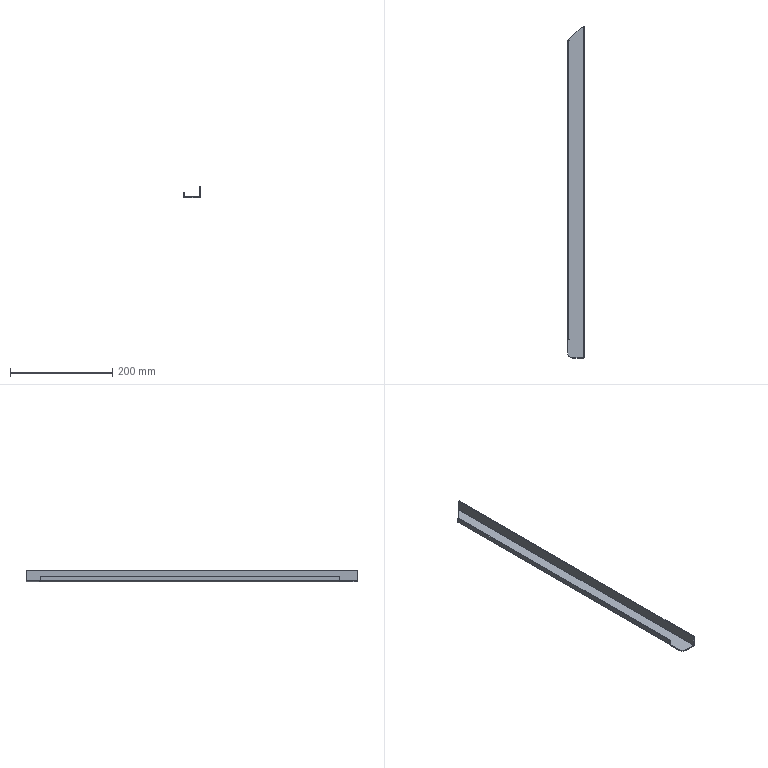Part | STEP file | Rear Closing Plate Door Frame Left | 1 solid | 25 faces | box 32 x 650 x 22 mm | volume 74925 mm3 | plane 17 | cylinder 7 | spline 1 | commonest cylinder face diameters 0.2 x4 4.2 x2 20 x1
STEP:
#1=CARTESIAN_POINT('',(677.249,-292.608,2.));
#2=VERTEX_POINT('',#1);
#3=CARTESIAN_POINT('',(667.249,-282.608,2.));
#4=VERTEX_POINT('',#3);
#5=CARTESIAN_POINT('',(677.249,-282.608,2.));
#6=DIRECTION('',(0.,0.,-1.));
#7=DIRECTION('',(-1.,0.,0.));
#8=AXIS2_PLACEMENT_3D('',#5,#6,#7);
#9=CIRCLE('',#8,10.);
#10=EDGE_CURVE('',#2,#4,#9,.T.);
#11=ORIENTED_EDGE('',*,*,#10,.F.);
#12=CARTESIAN_POINT('',(697.149,-292.608,2.));
#13=VERTEX_POINT('',#12);
#14=CARTESIAN_POINT('',(0.,-292.608,2.));
#15=DIRECTION('',(-1.,0.,0.));
#16=VECTOR('',#15,1000.);
#17=LINE('',#14,#16);
#18=EDGE_CURVE('',#13,#2,#17,.T.);
#19=ORIENTED_EDGE('',*,*,#18,.F.);
#20=CARTESIAN_POINT('',(697.149,357.299,2.));
#21=VERTEX_POINT('',#20);
#22=CARTESIAN_POINT('',(697.149,0.,2.));
#23=DIRECTION('',(0.,-1.,0.));
#24=VECTOR('',#23,1000.);
#25=LINE('',#22,#24);
#26=EDGE_CURVE('',#21,#13,#25,.T.);
#27=ORIENTED_EDGE('',*,*,#26,.F.);
#28=CARTESIAN_POINT('',(669.249,331.392,2.));
#29=VERTEX_POINT('',#28);
#30=CARTESIAN_POINT('',(669.249,331.392,2.));
#31=DIRECTION('',(0.7328,0.6805,0.));
#32=VECTOR('',#31,1000.);
#33=LINE('',#30,#32);
#34=EDGE_CURVE('',#29,#21,#33,.T.);
#35=ORIENTED_EDGE('',*,*,#34,.F.);
#36=CARTESIAN_POINT('',(669.249,329.592,2.));
#37=VERTEX_POINT('',#36);
#38=CARTESIAN_POINT('',(669.249,0.,2.));
#39=DIRECTION('',(0.,1.,0.));
#40=VECTOR('',#39,1000.);
#41=LINE('',#38,#40);
#42=EDGE_CURVE('',#37,#29,#41,.T.);
#43=ORIENTED_EDGE('',*,*,#42,.F.);
#44=CARTESIAN_POINT('',(669.549,329.592,2.));
#45=VERTEX_POINT('',#44);
#46=CARTESIAN_POINT('',(0.,329.592,2.));
#47=DIRECTION('',(-1.,0.,0.));
#48=VECTOR('',#47,1000.);
#49=LINE('',#46,#48);
#50=EDGE_CURVE('',#45,#37,#49,.T.);
#51=ORIENTED_EDGE('',*,*,#50,.F.);
#52=CARTESIAN_POINT('',(669.549,329.392,2.));
#53=VERTEX_POINT('',#52);
#54=CARTESIAN_POINT('',(669.549,329.492,2.));
#55=DIRECTION('',(0.,0.,-1.));
#56=DIRECTION('',(-1.,0.,0.));
#57=AXIS2_PLACEMENT_3D('',#54,#55,#56);
#58=CIRCLE('',#57,0.1);
#59=EDGE_CURVE('',#45,#53,#58,.T.);
#60=ORIENTED_EDGE('',*,*,#59,.T.);
#61=CARTESIAN_POINT('',(669.349,329.392,2.));
#62=VERTEX_POINT('',#61);
#63=CARTESIAN_POINT('',(0.,329.392,2.));
#64=DIRECTION('',(1.,0.,0.));
#65=VECTOR('',#64,1000.);
#66=LINE('',#63,#65);
#67=EDGE_CURVE('',#62,#53,#66,.T.);
#68=ORIENTED_EDGE('',*,*,#67,.F.);
#69=CARTESIAN_POINT('',(669.349,-256.608,2.));
#70=VERTEX_POINT('',#69);
#71=CARTESIAN_POINT('',(669.349,0.,2.));
#72=DIRECTION('',(0.,1.,0.));
#73=VECTOR('',#72,1000.);
#74=LINE('',#71,#73);
#75=EDGE_CURVE('',#70,#62,#74,.T.);
#76=ORIENTED_EDGE('',*,*,#75,.F.);
#77=CARTESIAN_POINT('',(669.549,-256.608,2.));
#78=VERTEX_POINT('',#77);
#79=CARTESIAN_POINT('',(0.,-256.608,2.));
#80=DIRECTION('',(-1.,0.,0.));
#81=VECTOR('',#80,1000.);
#82=LINE('',#79,#81);
#83=EDGE_CURVE('',#78,#70,#82,.T.);
#84=ORIENTED_EDGE('',*,*,#83,.F.);
#85=CARTESIAN_POINT('',(669.549,-256.808,2.));
#86=VERTEX_POINT('',#85);
#87=CARTESIAN_POINT('',(669.549,-256.708,2.));
#88=DIRECTION('',(0.,0.,-1.));
#89=DIRECTION('',(-1.,0.,0.));
#90=AXIS2_PLACEMENT_3D('',#87,#88,#89);
#91=CIRCLE('',#90,0.1);
#92=EDGE_CURVE('',#78,#86,#91,.T.);
#93=ORIENTED_EDGE('',*,*,#92,.T.);
#94=CARTESIAN_POINT('',(667.249,-256.808,2.));
#95=VERTEX_POINT('',#94);
#96=CARTESIAN_POINT('',(0.,-256.808,2.));
#97=DIRECTION('',(1.,0.,0.));
#98=VECTOR('',#97,1000.);
#99=LINE('',#96,#98);
#100=EDGE_CURVE('',#95,#86,#99,.T.);
#101=ORIENTED_EDGE('',*,*,#100,.F.);
#102=CARTESIAN_POINT('',(667.249,0.,2.));
#103=DIRECTION('',(0.,1.,0.));
#104=VECTOR('',#103,1000.);
#105=LINE('',#102,#104);
#106=EDGE_CURVE('',#4,#95,#105,.T.);
#107=ORIENTED_EDGE('',*,*,#106,.F.);
#108=EDGE_LOOP('',(#11,#19,#27,#35,#43,#51,#60,#68,#76,#84,#93,#101,#107));
#109=FACE_OUTER_BOUND('',#108,.T.);
#110=CARTESIAN_POINT('',(0.,0.,2.));
#111=DIRECTION('',(0.,0.,-1.));
#112=DIRECTION('',(-1.,0.,0.));
#113=AXIS2_PLACEMENT_3D('',#110,#111,#112);
#114=PLANE('',#113);
#115=ADVANCED_FACE('',(#109),#114,.F.);
#116=CARTESIAN_POINT('',(667.249,-282.608,0.));
#117=VERTEX_POINT('',#116);
#118=CARTESIAN_POINT('',(667.249,-282.608,1301.189));
#119=DIRECTION('',(0.,0.,-1.));
#120=VECTOR('',#119,1000.);
#121=LINE('',#118,#120);
#122=EDGE_CURVE('',#4,#117,#121,.T.);
#123=ORIENTED_EDGE('',*,*,#122,.F.);
#124=ORIENTED_EDGE('',*,*,#106,.T.);
#125=CARTESIAN_POINT('',(667.249,-256.808,0.));
#126=VERTEX_POINT('',#125);
#127=CARTESIAN_POINT('',(667.249,-256.808,1301.189));
#128=DIRECTION('',(0.,0.,1.));
#129=VECTOR('',#128,1000.);
#130=LINE('',#127,#129);
#131=EDGE_CURVE('',#126,#95,#130,.T.);
#132=ORIENTED_EDGE('',*,*,#131,.F.);
#133=CARTESIAN_POINT('',(667.249,0.,0.));
#134=DIRECTION('',(0.,1.,0.));
#135=VECTOR('',#134,1000.);
#136=LINE('',#133,#135);
#137=EDGE_CURVE('',#117,#126,#136,.T.);
#138=ORIENTED_EDGE('',*,*,#137,.F.);
#139=EDGE_LOOP('',(#123,#124,#132,#138));
#140=FACE_OUTER_BOUND('',#139,.T.);
#141=CARTESIAN_POINT('',(667.249,0.,1301.189));
#142=DIRECTION('',(1.,0.,0.));
#143=DIRECTION('',(0.,0.,-1.));
#144=AXIS2_PLACEMENT_3D('',#141,#142,#143);
#145=PLANE('',#144);
#146=ADVANCED_FACE('',(#140),#145,.F.);
#147=CARTESIAN_POINT('',(677.249,-292.608,0.));
#148=VERTEX_POINT('',#147);
#149=CARTESIAN_POINT('',(677.249,-282.608,0.));
#150=DIRECTION('',(0.,0.,1.));
#151=DIRECTION('',(-1.,0.,0.));
#152=AXIS2_PLACEMENT_3D('',#149,#150,#151);
#153=CIRCLE('',#152,10.);
#154=EDGE_CURVE('',#117,#148,#153,.T.);
#155=ORIENTED_EDGE('',*,*,#154,.T.);
#156=CARTESIAN_POINT('',(677.249,-292.608,1301.189));
#157=DIRECTION('',(0.,0.,1.));
#158=VECTOR('',#157,1000.);
#159=LINE('',#156,#158);
#160=EDGE_CURVE('',#148,#2,#159,.T.);
#161=ORIENTED_EDGE('',*,*,#160,.T.);
#162=ORIENTED_EDGE('',*,*,#10,.T.);
#163=ORIENTED_EDGE('',*,*,#122,.T.);
#164=EDGE_LOOP('',(#155,#161,#162,#163));
#165=FACE_OUTER_BOUND('',#164,.T.);
#166=CARTESIAN_POINT('',(677.249,-282.608,1301.189));
#167=DIRECTION('',(0.,0.,-1.));
#168=DIRECTION('',(-1.,0.,0.));
#169=AXIS2_PLACEMENT_3D('',#166,#167,#168);
#170=CYLINDRICAL_SURFACE('',#169,10.);
#171=ADVANCED_FACE('',(#165),#170,.T.);
#172=ORIENTED_EDGE('',*,*,#160,.F.);
#173=CARTESIAN_POINT('',(697.149,-292.608,0.));
#174=VERTEX_POINT('',#173);
#175=CARTESIAN_POINT('',(0.,-292.608,0.));
#176=DIRECTION('',(-1.,0.,0.));
#177=VECTOR('',#176,1000.);
#178=LINE('',#175,#177);
#179=EDGE_CURVE('',#174,#148,#178,.T.);
#180=ORIENTED_EDGE('',*,*,#179,.F.);
#181=CARTESIAN_POINT('',(699.249,-292.608,2.1));
#182=VERTEX_POINT('',#181);
#183=CARTESIAN_POINT('',(697.149,-292.608,2.1));
#184=DIRECTION('',(0.,-1.,0.));
#185=DIRECTION('',(-1.,0.,0.));
#186=AXIS2_PLACEMENT_3D('',#183,#184,#185);
#187=CIRCLE('',#186,2.1);
#188=EDGE_CURVE('',#174,#182,#187,.T.);
#189=ORIENTED_EDGE('',*,*,#188,.T.);
#190=CARTESIAN_POINT('',(699.249,-292.608,22.));
#191=VERTEX_POINT('',#190);
#192=CARTESIAN_POINT('',(699.249,-292.608,22.));
#193=DIRECTION('',(0.,0.,1.));
#194=VECTOR('',#193,1000.);
#195=LINE('',#192,#194);
#196=EDGE_CURVE('',#182,#191,#195,.T.);
#197=ORIENTED_EDGE('',*,*,#196,.T.);
#198=CARTESIAN_POINT('',(697.249,-292.608,22.));
#199=VERTEX_POINT('',#198);
#200=CARTESIAN_POINT('',(-601.36,-292.608,22.));
#201=DIRECTION('',(-1.,0.,0.));
#202=VECTOR('',#201,1000.);
#203=LINE('',#200,#202);
#204=EDGE_CURVE('',#191,#199,#203,.T.);
#205=ORIENTED_EDGE('',*,*,#204,.T.);
#206=CARTESIAN_POINT('',(697.249,-292.608,2.1));
#207=VERTEX_POINT('',#206);
#208=CARTESIAN_POINT('',(697.249,-292.608,22.));
#209=DIRECTION('',(0.,0.,1.));
#210=VECTOR('',#209,1000.);
#211=LINE('',#208,#210);
#212=EDGE_CURVE('',#207,#199,#211,.T.);
#213=ORIENTED_EDGE('',*,*,#212,.F.);
#214=CARTESIAN_POINT('',(697.149,-292.608,2.1));
#215=DIRECTION('',(0.,1.,0.));
#216=DIRECTION('',(-1.,0.,0.));
#217=AXIS2_PLACEMENT_3D('',#214,#215,#216);
#218=CIRCLE('',#217,0.1);
#219=EDGE_CURVE('',#207,#13,#218,.T.);
#220=ORIENTED_EDGE('',*,*,#219,.T.);
#221=ORIENTED_EDGE('',*,*,#18,.T.);
#222=EDGE_LOOP('',(#172,#180,#189,#197,#205,#213,#220,#221));
#223=FACE_OUTER_BOUND('',#222,.T.);
#224=CARTESIAN_POINT('',(0.,-292.608,1301.189));
#225=DIRECTION('',(0.,1.,0.));
#226=DIRECTION('',(0.,0.,1.));
#227=AXIS2_PLACEMENT_3D('',#224,#225,#226);
#228=PLANE('',#227);
#229=ADVANCED_FACE('',(#223),#228,.F.);
#230=ORIENTED_EDGE('',*,*,#219,.F.);
#231=CARTESIAN_POINT('',(697.249,357.392,2.1));
#232=VERTEX_POINT('',#231);
#233=CARTESIAN_POINT('',(697.249,-945.215,2.1));
#234=DIRECTION('',(0.,-1.,0.));
#235=VECTOR('',#234,1000.);
#236=LINE('',#233,#235);
#237=EDGE_CURVE('',#232,#207,#236,.T.);
#238=ORIENTED_EDGE('',*,*,#237,.F.);
#239=CARTESIAN_POINT('',(697.161,357.392,2.001));
#240=VERTEX_POINT('',#239);
#241=CARTESIAN_POINT('',(697.149,357.392,2.1));
#242=DIRECTION('',(0.,-1.,0.));
#243=DIRECTION('',(-1.,0.,0.));
#244=AXIS2_PLACEMENT_3D('',#241,#242,#243);
#245=CIRCLE('',#244,0.1);
#246=EDGE_CURVE('',#240,#232,#245,.T.);
#247=ORIENTED_EDGE('',*,*,#246,.F.);
#248=CARTESIAN_POINT('',(697.149,357.299,2.));
#249=CARTESIAN_POINT('',(697.153,357.33,2.));
#250=CARTESIAN_POINT('',(697.157,357.361,2.));
#251=CARTESIAN_POINT('',(697.161,357.392,2.001));
#252=B_SPLINE_CURVE_WITH_KNOTS('',3,(#248,#249,#250,#251),.UNSPECIFIED.,.F.,.F.,(4,4),(0.,1.),.UNSPECIFIED.);
#253=EDGE_CURVE('',#21,#240,#252,.T.);
#254=ORIENTED_EDGE('',*,*,#253,.F.);
#255=ORIENTED_EDGE('',*,*,#26,.T.);
#256=EDGE_LOOP('',(#230,#238,#247,#254,#255));
#257=FACE_OUTER_BOUND('',#256,.T.);
#258=CARTESIAN_POINT('',(697.149,-945.215,2.1));
#259=DIRECTION('',(0.,1.,0.));
#260=DIRECTION('',(-1.,0.,0.));
#261=AXIS2_PLACEMENT_3D('',#258,#259,#260);
#262=CYLINDRICAL_SURFACE('',#261,0.1);
#263=ADVANCED_FACE('',(#257),#262,.F.);
#264=CARTESIAN_POINT('',(669.249,331.392,0.));
#265=VERTEX_POINT('',#264);
#266=CARTESIAN_POINT('',(669.249,331.392,1301.189));
#267=DIRECTION('',(0.,0.,-1.));
#268=VECTOR('',#267,1000.);
#269=LINE('',#266,#268);
#270=EDGE_CURVE('',#29,#265,#269,.T.);
#271=ORIENTED_EDGE('',*,*,#270,.F.);
#272=ORIENTED_EDGE('',*,*,#34,.T.);
#273=CARTESIAN_POINT('',(697.149,357.299,0.));
#274=VERTEX_POINT('',#273);
#275=CARTESIAN_POINT('',(697.149,357.299,1301.189));
#276=DIRECTION('',(0.,0.,1.));
#277=VECTOR('',#276,1000.);
#278=LINE('',#275,#277);
#279=EDGE_CURVE('',#274,#21,#278,.T.);
#280=ORIENTED_EDGE('',*,*,#279,.F.);
#281=CARTESIAN_POINT('',(144.63,-155.755,0.));
#282=DIRECTION('',(0.7328,0.6805,0.));
#283=VECTOR('',#282,1000.);
#284=LINE('',#281,#283);
#285=EDGE_CURVE('',#265,#274,#284,.T.);
#286=ORIENTED_EDGE('',*,*,#285,.F.);
#287=EDGE_LOOP('',(#271,#272,#280,#286));
#288=FACE_OUTER_BOUND('',#287,.T.);
#289=CARTESIAN_POINT('',(144.63,-155.755,1301.189));
#290=DIRECTION('',(0.6805,-0.7328,0.));
#291=DIRECTION('',(0.7328,0.6805,0.));
#292=AXIS2_PLACEMENT_3D('',#289,#290,#291);
#293=PLANE('',#292);
#294=ADVANCED_FACE('',(#288),#293,.F.);
#295=CARTESIAN_POINT('',(669.249,329.592,0.));
#296=VERTEX_POINT('',#295);
#297=CARTESIAN_POINT('',(669.249,329.592,1301.189));
#298=DIRECTION('',(0.,0.,-1.));
#299=VECTOR('',#298,1000.);
#300=LINE('',#297,#299);
#301=EDGE_CURVE('',#37,#296,#300,.T.);
#302=ORIENTED_EDGE('',*,*,#301,.F.);
#303=ORIENTED_EDGE('',*,*,#42,.T.);
#304=ORIENTED_EDGE('',*,*,#270,.T.);
#305=CARTESIAN_POINT('',(669.249,0.,0.));
#306=DIRECTION('',(0.,1.,0.));
#307=VECTOR('',#306,1000.);
#308=LINE('',#305,#307);
#309=EDGE_CURVE('',#296,#265,#308,.T.);
#310=ORIENTED_EDGE('',*,*,#309,.F.);
#311=EDGE_LOOP('',(#302,#303,#304,#310));
#312=FACE_OUTER_BOUND('',#311,.T.);
#313=CARTESIAN_POINT('',(669.249,0.,1301.189));
#314=DIRECTION('',(1.,0.,0.));
#315=DIRECTION('',(0.,1.,0.));
#316=AXIS2_PLACEMENT_3D('',#313,#314,#315);
#317=PLANE('',#316);
#318=ADVANCED_FACE('',(#312),#317,.F.);
#319=CARTESIAN_POINT('',(669.249,329.392,2.1));
#320=VERTEX_POINT('',#319);
#321=CARTESIAN_POINT('',(669.349,329.392,2.1));
#322=DIRECTION('',(0.,-1.,0.));
#323=DIRECTION('',(0.,0.,-1.));
#324=AXIS2_PLACEMENT_3D('',#321,#322,#323);
#325=CIRCLE('',#324,0.1);
#326=EDGE_CURVE('',#320,#62,#325,.T.);
#327=ORIENTED_EDGE('',*,*,#326,.F.);
#328=CARTESIAN_POINT('',(669.249,-256.608,2.1));
#329=VERTEX_POINT('',#328);
#330=CARTESIAN_POINT('',(669.249,980.944,2.1));
#331=DIRECTION('',(0.,1.,0.));
#332=VECTOR('',#331,1000.);
#333=LINE('',#330,#332);
#334=EDGE_CURVE('',#329,#320,#333,.T.);
#335=ORIENTED_EDGE('',*,*,#334,.F.);
#336=CARTESIAN_POINT('',(669.349,-256.608,2.1));
#337=DIRECTION('',(0.,1.,0.));
#338=DIRECTION('',(0.,0.,-1.));
#339=AXIS2_PLACEMENT_3D('',#336,#337,#338);
#340=CIRCLE('',#339,0.1);
#341=EDGE_CURVE('',#70,#329,#340,.T.);
#342=ORIENTED_EDGE('',*,*,#341,.F.);
#343=ORIENTED_EDGE('',*,*,#75,.T.);
#344=EDGE_LOOP('',(#327,#335,#342,#343));
#345=FACE_OUTER_BOUND('',#344,.T.);
#346=CARTESIAN_POINT('',(669.349,980.944,2.1));
#347=DIRECTION('',(0.,-1.,0.));
#348=DIRECTION('',(0.,0.,-1.));
#349=AXIS2_PLACEMENT_3D('',#346,#347,#348);
#350=CYLINDRICAL_SURFACE('',#349,0.1);
#351=ADVANCED_FACE('',(#345),#350,.F.);
#352=ORIENTED_EDGE('',*,*,#131,.T.);
#353=ORIENTED_EDGE('',*,*,#100,.T.);
#354=CARTESIAN_POINT('',(669.549,-256.808,0.));
#355=VERTEX_POINT('',#354);
#356=CARTESIAN_POINT('',(669.549,-256.808,1301.189));
#357=DIRECTION('',(0.,0.,-1.));
#358=VECTOR('',#357,1000.);
#359=LINE('',#356,#358);
#360=EDGE_CURVE('',#86,#355,#359,.T.);
#361=ORIENTED_EDGE('',*,*,#360,.T.);
#362=CARTESIAN_POINT('',(0.,-256.808,0.));
#363=DIRECTION('',(-1.,0.,0.));
#364=VECTOR('',#363,1000.);
#365=LINE('',#362,#364);
#366=EDGE_CURVE('',#355,#126,#365,.T.);
#367=ORIENTED_EDGE('',*,*,#366,.T.);
#368=EDGE_LOOP('',(#352,#353,#361,#367));
#369=FACE_OUTER_BOUND('',#368,.T.);
#370=CARTESIAN_POINT('',(0.,-256.808,1301.189));
#371=DIRECTION('',(0.,1.,0.));
#372=DIRECTION('',(0.,0.,1.));
#373=AXIS2_PLACEMENT_3D('',#370,#371,#372);
#374=PLANE('',#373);
#375=ADVANCED_FACE('',(#369),#374,.T.);
#376=ORIENTED_EDGE('',*,*,#285,.T.);
#377=CARTESIAN_POINT('',(697.149,0.,0.));
#378=DIRECTION('',(0.,-1.,0.));
#379=VECTOR('',#378,1000.);
#380=LINE('',#377,#379);
#381=EDGE_CURVE('',#274,#174,#380,.T.);
#382=ORIENTED_EDGE('',*,*,#381,.T.);
#383=ORIENTED_EDGE('',*,*,#179,.T.);
#384=ORIENTED_EDGE('',*,*,#154,.F.);
#385=ORIENTED_EDGE('',*,*,#137,.T.);
#386=ORIENTED_EDGE('',*,*,#366,.F.);
#387=CARTESIAN_POINT('',(669.549,-256.608,0.));
#388=VERTEX_POINT('',#387);
#389=CARTESIAN_POINT('',(669.549,-256.708,0.));
#390=DIRECTION('',(0.,0.,1.));
#391=DIRECTION('',(-1.,0.,0.));
#392=AXIS2_PLACEMENT_3D('',#389,#390,#391);
#393=CIRCLE('',#392,0.1);
#394=EDGE_CURVE('',#355,#388,#393,.T.);
#395=ORIENTED_EDGE('',*,*,#394,.T.);
#396=CARTESIAN_POINT('',(669.349,-256.608,0.));
#397=VERTEX_POINT('',#396);
#398=CARTESIAN_POINT('',(0.,-256.608,0.));
#399=DIRECTION('',(1.,0.,0.));
#400=VECTOR('',#399,1000.);
#401=LINE('',#398,#400);
#402=EDGE_CURVE('',#397,#388,#401,.T.);
#403=ORIENTED_EDGE('',*,*,#402,.F.);
#404=CARTESIAN_POINT('',(669.349,329.392,0.));
#405=VERTEX_POINT('',#404);
#406=CARTESIAN_POINT('',(669.349,0.,0.));
#407=DIRECTION('',(0.,1.,0.));
#408=VECTOR('',#407,1000.);
#409=LINE('',#406,#408);
#410=EDGE_CURVE('',#397,#405,#409,.T.);
#411=ORIENTED_EDGE('',*,*,#410,.T.);
#412=CARTESIAN_POINT('',(669.549,329.392,0.));
#413=VERTEX_POINT('',#412);
#414=CARTESIAN_POINT('',(0.,329.392,0.));
#415=DIRECTION('',(-1.,0.,0.));
#416=VECTOR('',#415,1000.);
#417=LINE('',#414,#416);
#418=EDGE_CURVE('',#413,#405,#417,.T.);
#419=ORIENTED_EDGE('',*,*,#418,.F.);
#420=CARTESIAN_POINT('',(669.549,329.592,0.));
#421=VERTEX_POINT('',#420);
#422=CARTESIAN_POINT('',(669.549,329.492,0.));
#423=DIRECTION('',(0.,0.,1.));
#424=DIRECTION('',(-1.,0.,0.));
#425=AXIS2_PLACEMENT_3D('',#422,#423,#424);
#426=CIRCLE('',#425,0.1);
#427=EDGE_CURVE('',#413,#421,#426,.T.);
#428=ORIENTED_EDGE('',*,*,#427,.T.);
#429=CARTESIAN_POINT('',(0.,329.592,0.));
#430=DIRECTION('',(-1.,0.,0.));
#431=VECTOR('',#430,1000.);
#432=LINE('',#429,#431);
#433=EDGE_CURVE('',#421,#296,#432,.T.);
#434=ORIENTED_EDGE('',*,*,#433,.T.);
#435=ORIENTED_EDGE('',*,*,#309,.T.);
#436=EDGE_LOOP('',(#376,#382,#383,#384,#385,#386,#395,#403,#411,#419,#428,#434,#435));
#437=FACE_OUTER_BOUND('',#436,.T.);
#438=CARTESIAN_POINT('',(0.,0.,0.));
#439=DIRECTION('',(0.,0.,-1.));
#440=DIRECTION('',(-1.,0.,0.));
#441=AXIS2_PLACEMENT_3D('',#438,#439,#440);
#442=PLANE('',#441);
#443=ADVANCED_FACE('',(#437),#442,.T.);
#444=CARTESIAN_POINT('',(697.249,357.392,22.));
#445=VERTEX_POINT('',#444);
#446=CARTESIAN_POINT('',(697.249,359.392,22.));
#447=DIRECTION('',(0.,1.,0.));
#448=VECTOR('',#447,1000.);
#449=LINE('',#446,#448);
#450=EDGE_CURVE('',#199,#445,#449,.T.);
#451=ORIENTED_EDGE('',*,*,#450,.T.);
#452=CARTESIAN_POINT('',(697.249,357.392,22.));
#453=DIRECTION('',(0.,0.,-1.));
#454=VECTOR('',#453,1000.);
#455=LINE('',#452,#454);
#456=EDGE_CURVE('',#445,#232,#455,.T.);
#457=ORIENTED_EDGE('',*,*,#456,.T.);
#458=ORIENTED_EDGE('',*,*,#237,.T.);
#459=ORIENTED_EDGE('',*,*,#212,.T.);
#460=EDGE_LOOP('',(#451,#457,#458,#459));
#461=FACE_OUTER_BOUND('',#460,.T.);
#462=CARTESIAN_POINT('',(697.249,359.392,22.));
#463=DIRECTION('',(-1.,0.,0.));
#464=DIRECTION('',(0.,-1.,0.));
#465=AXIS2_PLACEMENT_3D('',#462,#463,#464);
#466=PLANE('',#465);
#467=ADVANCED_FACE('',(#461),#466,.T.);
#468=CARTESIAN_POINT('',(697.398,357.392,0.01486));
#469=VERTEX_POINT('',#468);
#470=CARTESIAN_POINT('',(697.398,357.392,0.01486));
#471=CARTESIAN_POINT('',(697.316,357.361,0.004966));
#472=CARTESIAN_POINT('',(697.232,357.33,0.));
#473=CARTESIAN_POINT('',(697.149,357.299,0.));
#474=B_SPLINE_CURVE_WITH_KNOTS('',3,(#470,#471,#472,#473),.UNSPECIFIED.,.F.,.F.,(4,4),(0.,1.),.UNSPECIFIED.);
#475=EDGE_CURVE('',#469,#274,#474,.T.);
#476=ORIENTED_EDGE('',*,*,#475,.T.);
#477=ORIENTED_EDGE('',*,*,#279,.T.);
#478=ORIENTED_EDGE('',*,*,#253,.T.);
#479=CARTESIAN_POINT('',(697.279,357.392,1.008));
#480=DIRECTION('',(0.1188,0.,-0.9929));
#481=VECTOR('',#480,1000.);
#482=LINE('',#479,#481);
#483=EDGE_CURVE('',#240,#469,#482,.T.);
#484=ORIENTED_EDGE('',*,*,#483,.T.);
#485=EDGE_LOOP('',(#476,#477,#478,#484));
#486=FACE_OUTER_BOUND('',#485,.T.);
#487=CARTESIAN_POINT('',(697.149,357.299,0.));
#488=CARTESIAN_POINT('',(697.232,357.33,0.));
#489=CARTESIAN_POINT('',(697.316,357.361,0.004966));
#490=CARTESIAN_POINT('',(697.398,357.392,0.01486));
#491=CARTESIAN_POINT('',(697.149,357.299,2.));
#492=CARTESIAN_POINT('',(697.153,357.33,2.));
#493=CARTESIAN_POINT('',(697.157,357.361,2.));
#494=CARTESIAN_POINT('',(697.161,357.392,2.001));
#495=B_SPLINE_SURFACE_WITH_KNOTS('',1,3,((#487,#488,#489,#490),(#491,#492,#493,#494)),.UNSPECIFIED.,.F.,.F.,.F.,(2,2),(4,4),(0.,1.),(0.,1.),.UNSPECIFIED.);
#496=ADVANCED_FACE('',(#486),#495,.T.);
#497=CARTESIAN_POINT('',(669.549,329.592,1301.189));
#498=DIRECTION('',(0.,0.,1.));
#499=VECTOR('',#498,1000.);
#500=LINE('',#497,#499);
#501=EDGE_CURVE('',#421,#45,#500,.T.);
#502=ORIENTED_EDGE('',*,*,#501,.T.);
#503=ORIENTED_EDGE('',*,*,#50,.T.);
#504=ORIENTED_EDGE('',*,*,#301,.T.);
#505=ORIENTED_EDGE('',*,*,#433,.F.);
#506=EDGE_LOOP('',(#502,#503,#504,#505));
#507=FACE_OUTER_BOUND('',#506,.T.);
#508=CARTESIAN_POINT('',(0.,329.592,1301.189));
#509=DIRECTION('',(0.,-1.,0.));
#510=DIRECTION('',(0.,0.,-1.));
#511=AXIS2_PLACEMENT_3D('',#508,#509,#510);
#512=PLANE('',#511);
#513=ADVANCED_FACE('',(#507),#512,.T.);
#514=ORIENTED_EDGE('',*,*,#334,.T.);
#515=CARTESIAN_POINT('',(669.249,329.392,10.));
#516=VERTEX_POINT('',#515);
#517=CARTESIAN_POINT('',(669.249,329.392,22.));
#518=DIRECTION('',(0.,0.,-1.));
#519=VECTOR('',#518,1000.);
#520=LINE('',#517,#519);
#521=EDGE_CURVE('',#516,#320,#520,.T.);
#522=ORIENTED_EDGE('',*,*,#521,.F.);
#523=CARTESIAN_POINT('',(669.249,-256.608,10.));
#524=VERTEX_POINT('',#523);
#525=CARTESIAN_POINT('',(669.249,329.392,10.));
#526=DIRECTION('',(0.,1.,0.));
#527=VECTOR('',#526,1000.);
#528=LINE('',#525,#527);
#529=EDGE_CURVE('',#524,#516,#528,.T.);
#530=ORIENTED_EDGE('',*,*,#529,.F.);
#531=CARTESIAN_POINT('',(669.249,-256.608,22.));
#532=DIRECTION('',(0.,0.,1.));
#533=VECTOR('',#532,1000.);
#534=LINE('',#531,#533);
#535=EDGE_CURVE('',#329,#524,#534,.T.);
#536=ORIENTED_EDGE('',*,*,#535,.F.);
#537=EDGE_LOOP('',(#514,#522,#530,#536));
#538=FACE_OUTER_BOUND('',#537,.T.);
#539=CARTESIAN_POINT('',(669.249,329.392,22.));
#540=DIRECTION('',(-1.,0.,0.));
#541=DIRECTION('',(0.,-1.,0.));
#542=AXIS2_PLACEMENT_3D('',#539,#540,#541);
#543=PLANE('',#542);
#544=ADVANCED_FACE('',(#538),#543,.F.);
#545=ORIENTED_EDGE('',*,*,#360,.F.);
#546=ORIENTED_EDGE('',*,*,#92,.F.);
#547=CARTESIAN_POINT('',(669.549,-256.608,1301.189));
#548=DIRECTION('',(0.,0.,1.));
#549=VECTOR('',#548,1000.);
#550=LINE('',#547,#549);
#551=EDGE_CURVE('',#388,#78,#550,.T.);
#552=ORIENTED_EDGE('',*,*,#551,.F.);
#553=ORIENTED_EDGE('',*,*,#394,.F.);
#554=EDGE_LOOP('',(#545,#546,#552,#553));
#555=FACE_OUTER_BOUND('',#554,.T.);
#556=CARTESIAN_POINT('',(669.549,-256.708,1301.189));
#557=DIRECTION('',(0.,0.,-1.));
#558=DIRECTION('',(-1.,0.,0.));
#559=AXIS2_PLACEMENT_3D('',#556,#557,#558);
#560=CYLINDRICAL_SURFACE('',#559,0.1);
#561=ADVANCED_FACE('',(#555),#560,.F.);
#562=CARTESIAN_POINT('',(699.249,357.392,2.1));
#563=VERTEX_POINT('',#562);
#564=CARTESIAN_POINT('',(699.249,-945.215,2.1));
#565=DIRECTION('',(0.,-1.,0.));
#566=VECTOR('',#565,1000.);
#567=LINE('',#564,#566);
#568=EDGE_CURVE('',#563,#182,#567,.T.);
#569=ORIENTED_EDGE('',*,*,#568,.T.);
#570=ORIENTED_EDGE('',*,*,#188,.F.);
#571=ORIENTED_EDGE('',*,*,#381,.F.);
#572=ORIENTED_EDGE('',*,*,#475,.F.);
#573=CARTESIAN_POINT('',(697.149,357.392,2.1));
#574=DIRECTION('',(0.,-1.,0.));
#575=DIRECTION('',(-1.,0.,0.));
#576=AXIS2_PLACEMENT_3D('',#573,#574,#575);
#577=CIRCLE('',#576,2.1);
#578=EDGE_CURVE('',#469,#563,#577,.T.);
#579=ORIENTED_EDGE('',*,*,#578,.T.);
#580=EDGE_LOOP('',(#569,#570,#571,#572,#579));
#581=FACE_OUTER_BOUND('',#580,.T.);
#582=CARTESIAN_POINT('',(697.149,-945.215,2.1));
#583=DIRECTION('',(0.,1.,0.));
#584=DIRECTION('',(-1.,0.,0.));
#585=AXIS2_PLACEMENT_3D('',#582,#583,#584);
#586=CYLINDRICAL_SURFACE('',#585,2.1);
#587=ADVANCED_FACE('',(#581),#586,.T.);
#588=CARTESIAN_POINT('',(667.249,-256.608,2.1));
#589=VERTEX_POINT('',#588);
#590=CARTESIAN_POINT('',(667.249,329.392,2.1));
#591=VERTEX_POINT('',#590);
#592=CARTESIAN_POINT('',(667.249,980.944,2.1));
#593=DIRECTION('',(0.,1.,0.));
#594=VECTOR('',#593,1000.);
#595=LINE('',#592,#594);
#596=EDGE_CURVE('',#589,#591,#595,.T.);
#597=ORIENTED_EDGE('',*,*,#596,.T.);
#598=CARTESIAN_POINT('',(669.349,329.392,2.1));
#599=DIRECTION('',(0.,-1.,0.));
#600=DIRECTION('',(0.,0.,-1.));
#601=AXIS2_PLACEMENT_3D('',#598,#599,#600);
#602=CIRCLE('',#601,2.1);
#603=EDGE_CURVE('',#591,#405,#602,.T.);
#604=ORIENTED_EDGE('',*,*,#603,.T.);
#605=ORIENTED_EDGE('',*,*,#410,.F.);
#606=CARTESIAN_POINT('',(669.349,-256.608,2.1));
#607=DIRECTION('',(0.,1.,0.));
#608=DIRECTION('',(0.,0.,-1.));
#609=AXIS2_PLACEMENT_3D('',#606,#607,#608);
#610=CIRCLE('',#609,2.1);
#611=EDGE_CURVE('',#397,#589,#610,.T.);
#612=ORIENTED_EDGE('',*,*,#611,.T.);
#613=EDGE_LOOP('',(#597,#604,#605,#612));
#614=FACE_OUTER_BOUND('',#613,.T.);
#615=CARTESIAN_POINT('',(669.349,980.944,2.1));
#616=DIRECTION('',(0.,-1.,0.));
#617=DIRECTION('',(0.,0.,-1.));
#618=AXIS2_PLACEMENT_3D('',#615,#616,#617);
#619=CYLINDRICAL_SURFACE('',#618,2.1);
#620=ADVANCED_FACE('',(#614),#619,.T.);
#621=CARTESIAN_POINT('',(699.249,357.392,22.));
#622=VERTEX_POINT('',#621);
#623=CARTESIAN_POINT('',(699.249,357.392,22.));
#624=DIRECTION('',(0.,0.,1.));
#625=VECTOR('',#624,1000.);
#626=LINE('',#623,#625);
#627=EDGE_CURVE('',#563,#622,#626,.T.);
#628=ORIENTED_EDGE('',*,*,#627,.F.);
#629=ORIENTED_EDGE('',*,*,#578,.F.);
#630=ORIENTED_EDGE('',*,*,#483,.F.);
#631=ORIENTED_EDGE('',*,*,#246,.T.);
#632=ORIENTED_EDGE('',*,*,#456,.F.);
#633=CARTESIAN_POINT('',(-601.36,357.392,22.));
#634=DIRECTION('',(-1.,0.,0.));
#635=VECTOR('',#634,1000.);
#636=LINE('',#633,#635);
#637=EDGE_CURVE('',#622,#445,#636,.T.);
#638=ORIENTED_EDGE('',*,*,#637,.F.);
#639=EDGE_LOOP('',(#628,#629,#630,#631,#632,#638));
#640=FACE_OUTER_BOUND('',#639,.T.);
#641=CARTESIAN_POINT('',(-601.36,357.392,22.));
#642=DIRECTION('',(0.,-1.,0.));
#643=DIRECTION('',(1.,0.,0.));
#644=AXIS2_PLACEMENT_3D('',#641,#642,#643);
#645=PLANE('',#644);
#646=ADVANCED_FACE('',(#640),#645,.F.);
#647=CARTESIAN_POINT('',(699.249,0.,22.));
#648=DIRECTION('',(0.,-1.,0.));
#649=VECTOR('',#648,1000.);
#650=LINE('',#647,#649);
#651=EDGE_CURVE('',#622,#191,#650,.T.);
#652=ORIENTED_EDGE('',*,*,#651,.F.);
#653=ORIENTED_EDGE('',*,*,#637,.T.);
#654=ORIENTED_EDGE('',*,*,#450,.F.);
#655=ORIENTED_EDGE('',*,*,#204,.F.);
#656=EDGE_LOOP('',(#652,#653,#654,#655));
#657=FACE_OUTER_BOUND('',#656,.T.);
#658=CARTESIAN_POINT('',(-601.36,0.,22.));
#659=DIRECTION('',(0.,0.,-1.));
#660=DIRECTION('',(0.,1.,0.));
#661=AXIS2_PLACEMENT_3D('',#658,#659,#660);
#662=PLANE('',#661);
#663=ADVANCED_FACE('',(#657),#662,.F.);
#664=CARTESIAN_POINT('',(669.549,329.392,1301.189));
#665=DIRECTION('',(0.,0.,-1.));
#666=VECTOR('',#665,1000.);
#667=LINE('',#664,#666);
#668=EDGE_CURVE('',#53,#413,#667,.T.);
#669=ORIENTED_EDGE('',*,*,#668,.F.);
#670=ORIENTED_EDGE('',*,*,#59,.F.);
#671=ORIENTED_EDGE('',*,*,#501,.F.);
#672=ORIENTED_EDGE('',*,*,#427,.F.);
#673=EDGE_LOOP('',(#669,#670,#671,#672));
#674=FACE_OUTER_BOUND('',#673,.T.);
#675=CARTESIAN_POINT('',(669.549,329.492,1301.189));
#676=DIRECTION('',(0.,0.,-1.));
#677=DIRECTION('',(-1.,0.,0.));
#678=AXIS2_PLACEMENT_3D('',#675,#676,#677);
#679=CYLINDRICAL_SURFACE('',#678,0.1);
#680=ADVANCED_FACE('',(#674),#679,.F.);
#681=CARTESIAN_POINT('',(667.249,-256.608,10.));
#682=VERTEX_POINT('',#681);
#683=CARTESIAN_POINT('',(667.249,-256.608,22.));
#684=DIRECTION('',(0.,0.,1.));
#685=VECTOR('',#684,1000.);
#686=LINE('',#683,#685);
#687=EDGE_CURVE('',#589,#682,#686,.T.);
#688=ORIENTED_EDGE('',*,*,#687,.F.);
#689=ORIENTED_EDGE('',*,*,#611,.F.);
#690=ORIENTED_EDGE('',*,*,#402,.T.);
#691=ORIENTED_EDGE('',*,*,#551,.T.);
#692=ORIENTED_EDGE('',*,*,#83,.T.);
#693=ORIENTED_EDGE('',*,*,#341,.T.);
#694=ORIENTED_EDGE('',*,*,#535,.T.);
#695=CARTESIAN_POINT('',(1839.355,-256.608,10.));
#696=DIRECTION('',(1.,0.,0.));
#697=VECTOR('',#696,1000.);
#698=LINE('',#695,#697);
#699=EDGE_CURVE('',#682,#524,#698,.T.);
#700=ORIENTED_EDGE('',*,*,#699,.F.);
#701=EDGE_LOOP('',(#688,#689,#690,#691,#692,#693,#694,#700));
#702=FACE_OUTER_BOUND('',#701,.T.);
#703=CARTESIAN_POINT('',(1839.355,-256.608,22.));
#704=DIRECTION('',(0.,1.,0.));
#705=DIRECTION('',(0.,0.,1.));
#706=AXIS2_PLACEMENT_3D('',#703,#704,#705);
#707=PLANE('',#706);
#708=ADVANCED_FACE('',(#702),#707,.F.);
#709=CARTESIAN_POINT('',(667.249,329.392,10.));
#710=VERTEX_POINT('',#709);
#711=CARTESIAN_POINT('',(1839.355,329.392,10.));
#712=DIRECTION('',(1.,0.,0.));
#713=VECTOR('',#712,1000.);
#714=LINE('',#711,#713);
#715=EDGE_CURVE('',#710,#516,#714,.T.);
#716=ORIENTED_EDGE('',*,*,#715,.T.);
#717=ORIENTED_EDGE('',*,*,#521,.T.);
#718=ORIENTED_EDGE('',*,*,#326,.T.);
#719=ORIENTED_EDGE('',*,*,#67,.T.);
#720=ORIENTED_EDGE('',*,*,#668,.T.);
#721=ORIENTED_EDGE('',*,*,#418,.T.);
#722=ORIENTED_EDGE('',*,*,#603,.F.);
#723=CARTESIAN_POINT('',(667.249,329.392,22.));
#724=DIRECTION('',(0.,0.,1.));
#725=VECTOR('',#724,1000.);
#726=LINE('',#723,#725);
#727=EDGE_CURVE('',#591,#710,#726,.T.);
#728=ORIENTED_EDGE('',*,*,#727,.T.);
#729=EDGE_LOOP('',(#716,#717,#718,#719,#720,#721,#722,#728));
#730=FACE_OUTER_BOUND('',#729,.T.);
#731=CARTESIAN_POINT('',(1839.355,329.392,22.));
#732=DIRECTION('',(0.,1.,0.));
#733=DIRECTION('',(0.,0.,1.));
#734=AXIS2_PLACEMENT_3D('',#731,#732,#733);
#735=PLANE('',#734);
#736=ADVANCED_FACE('',(#730),#735,.T.);
#737=ORIENTED_EDGE('',*,*,#699,.T.);
#738=ORIENTED_EDGE('',*,*,#529,.T.);
#739=ORIENTED_EDGE('',*,*,#715,.F.);
#740=CARTESIAN_POINT('',(667.249,331.392,10.));
#741=DIRECTION('',(0.,-1.,0.));
#742=VECTOR('',#741,1000.);
#743=LINE('',#740,#742);
#744=EDGE_CURVE('',#710,#682,#743,.T.);
#745=ORIENTED_EDGE('',*,*,#744,.T.);
#746=EDGE_LOOP('',(#737,#738,#739,#745));
#747=FACE_OUTER_BOUND('',#746,.T.);
#748=CARTESIAN_POINT('',(1839.355,331.392,10.));
#749=DIRECTION('',(0.,0.,1.));
#750=DIRECTION('',(0.,-1.,0.));
#751=AXIS2_PLACEMENT_3D('',#748,#749,#750);
#752=PLANE('',#751);
#753=ADVANCED_FACE('',(#747),#752,.T.);
#754=ORIENTED_EDGE('',*,*,#568,.F.);
#755=ORIENTED_EDGE('',*,*,#627,.T.);
#756=ORIENTED_EDGE('',*,*,#651,.T.);
#757=ORIENTED_EDGE('',*,*,#196,.F.);
#758=EDGE_LOOP('',(#754,#755,#756,#757));
#759=FACE_OUTER_BOUND('',#758,.T.);
#760=CARTESIAN_POINT('',(699.249,359.392,22.));
#761=DIRECTION('',(-1.,0.,0.));
#762=DIRECTION('',(0.,-1.,0.));
#763=AXIS2_PLACEMENT_3D('',#760,#761,#762);
#764=PLANE('',#763);
#765=ADVANCED_FACE('',(#759),#764,.F.);
#766=ORIENTED_EDGE('',*,*,#744,.F.);
#767=ORIENTED_EDGE('',*,*,#727,.F.);
#768=ORIENTED_EDGE('',*,*,#596,.F.);
#769=ORIENTED_EDGE('',*,*,#687,.T.);
#770=EDGE_LOOP('',(#766,#767,#768,#769));
#771=FACE_OUTER_BOUND('',#770,.T.);
#772=CARTESIAN_POINT('',(667.249,329.392,22.));
#773=DIRECTION('',(-1.,0.,0.));
#774=DIRECTION('',(0.,-1.,0.));
#775=AXIS2_PLACEMENT_3D('',#772,#773,#774);
#776=PLANE('',#775);
#777=ADVANCED_FACE('',(#771),#776,.T.);
#778=CLOSED_SHELL('',(#115,#146,#171,#229,#263,#294,#318,#351,#375,#443,#467,#496,#513,#544,#561,#587,#620,#646,#663,#680,#708,#736,#753,#765,#777));
#779=MANIFOLD_SOLID_BREP('',#778);
#780=CARTESIAN_POINT('',(0.,0.,0.));
#781=DIRECTION('',(0.,0.,1.));
#782=DIRECTION('',(1.,0.,0.));
#783=AXIS2_PLACEMENT_3D('',#780,#781,#782);
#784=(LENGTH_UNIT()NAMED_UNIT(*)SI_UNIT(.MILLI.,.METRE.));
#785=UNCERTAINTY_MEASURE_WITH_UNIT(LENGTH_MEASURE(0.00001),#784,'','');
#786=(NAMED_UNIT(*)PLANE_ANGLE_UNIT()SI_UNIT($,.RADIAN.));
#787=(NAMED_UNIT(*)SI_UNIT($,.STERADIAN.)SOLID_ANGLE_UNIT());
#788=(GEOMETRIC_REPRESENTATION_CONTEXT(3)GLOBAL_UNCERTAINTY_ASSIGNED_CONTEXT((#785))GLOBAL_UNIT_ASSIGNED_CONTEXT((#784,#786,#787))REPRESENTATION_CONTEXT('',''));
#789=ADVANCED_BREP_SHAPE_REPRESENTATION('',(#779,#783),#788);